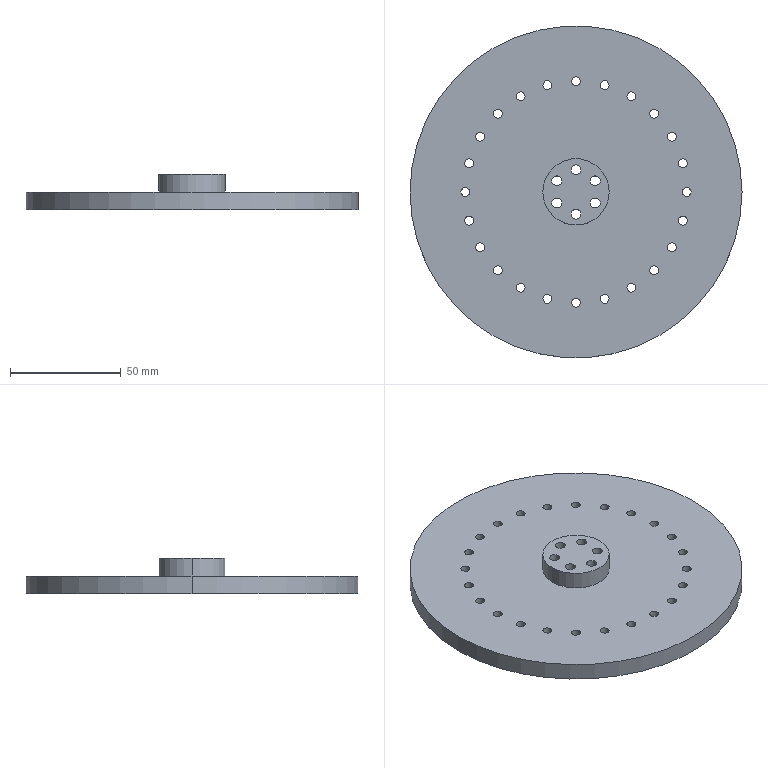Part | SolidWorks | features BaseBody 1 | 1 solid | 67 faces | box 150 x 150 x 16 mm | volume 143087 mm3 | cylinder 64 | plane 3 | commonest cylinder face diameters 4 x48 4.5 x12 30 x2 150 x2